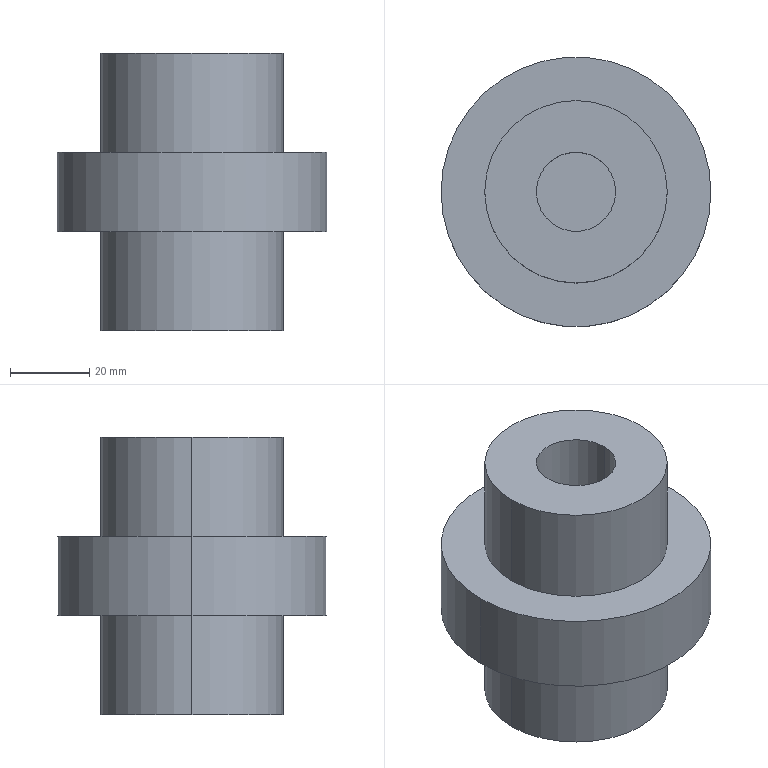Part | SolidWorks | features ICE 3, Extrusion 1, MirrorPattern 1 | 1 solid | 16 faces | box 68 x 68 x 70 mm | volume 136716 mm3 | cylinder 10 | plane 6 | commonest cylinder face diameters 46 x4 20 x2 32 x2 68 x2
STEP:
#1=CARTESIAN_POINT('',(16.,0.,-18.));
#2=VERTEX_POINT('',#1);
#3=CARTESIAN_POINT('',(-16.,0.,-18.));
#4=VERTEX_POINT('',#3);
#5=CARTESIAN_POINT('',(0.,0.,-18.));
#6=DIRECTION('',(0.,0.,-1.));
#7=DIRECTION('',(-1.,0.,0.));
#8=AXIS2_PLACEMENT_3D('',#5,#6,#7);
#9=CIRCLE('',#8,16.);
#10=EDGE_CURVE('',#2,#4,#9,.T.);
#11=ORIENTED_EDGE('',*,*,#10,.F.);
#12=CARTESIAN_POINT('',(16.,0.,-35.));
#13=VERTEX_POINT('',#12);
#14=CARTESIAN_POINT('',(16.,0.,-18.));
#15=DIRECTION('',(0.,0.,-1.));
#16=VECTOR('',#15,1000.);
#17=LINE('',#14,#16);
#18=EDGE_CURVE('',#2,#13,#17,.T.);
#19=ORIENTED_EDGE('',*,*,#18,.T.);
#20=CARTESIAN_POINT('',(-16.,0.,-35.));
#21=VERTEX_POINT('',#20);
#22=CARTESIAN_POINT('',(0.,0.,-35.));
#23=DIRECTION('',(0.,0.,-1.));
#24=DIRECTION('',(-1.,0.,0.));
#25=AXIS2_PLACEMENT_3D('',#22,#23,#24);
#26=CIRCLE('',#25,16.);
#27=EDGE_CURVE('',#13,#21,#26,.T.);
#28=ORIENTED_EDGE('',*,*,#27,.T.);
#29=CARTESIAN_POINT('',(-16.,0.,-18.));
#30=DIRECTION('',(0.,0.,-1.));
#31=VECTOR('',#30,1000.);
#32=LINE('',#29,#31);
#33=EDGE_CURVE('',#4,#21,#32,.T.);
#34=ORIENTED_EDGE('',*,*,#33,.F.);
#35=EDGE_LOOP('',(#11,#19,#28,#34));
#36=FACE_OUTER_BOUND('',#35,.T.);
#37=CARTESIAN_POINT('',(0.,0.,-18.));
#38=DIRECTION('',(0.,0.,-1.));
#39=DIRECTION('',(-1.,0.,0.));
#40=AXIS2_PLACEMENT_3D('',#37,#38,#39);
#41=CYLINDRICAL_SURFACE('',#40,16.);
#42=ADVANCED_FACE('',(#36),#41,.F.);
#43=CARTESIAN_POINT('',(-10.,0.,18.));
#44=VERTEX_POINT('',#43);
#45=CARTESIAN_POINT('',(10.,0.,18.));
#46=VERTEX_POINT('',#45);
#47=CARTESIAN_POINT('',(0.,0.,18.));
#48=DIRECTION('',(0.,0.,1.));
#49=DIRECTION('',(1.,0.,0.));
#50=AXIS2_PLACEMENT_3D('',#47,#48,#49);
#51=CIRCLE('',#50,10.);
#52=EDGE_CURVE('',#44,#46,#51,.T.);
#53=ORIENTED_EDGE('',*,*,#52,.F.);
#54=CARTESIAN_POINT('',(-10.,0.,35.));
#55=VERTEX_POINT('',#54);
#56=CARTESIAN_POINT('',(-10.,0.,18.));
#57=DIRECTION('',(0.,0.,1.));
#58=VECTOR('',#57,1000.);
#59=LINE('',#56,#58);
#60=EDGE_CURVE('',#44,#55,#59,.T.);
#61=ORIENTED_EDGE('',*,*,#60,.T.);
#62=CARTESIAN_POINT('',(10.,0.,35.));
#63=VERTEX_POINT('',#62);
#64=CARTESIAN_POINT('',(0.,0.,35.));
#65=DIRECTION('',(0.,0.,1.));
#66=DIRECTION('',(1.,0.,0.));
#67=AXIS2_PLACEMENT_3D('',#64,#65,#66);
#68=CIRCLE('',#67,10.);
#69=EDGE_CURVE('',#55,#63,#68,.T.);
#70=ORIENTED_EDGE('',*,*,#69,.T.);
#71=CARTESIAN_POINT('',(10.,0.,18.));
#72=DIRECTION('',(0.,0.,1.));
#73=VECTOR('',#72,1000.);
#74=LINE('',#71,#73);
#75=EDGE_CURVE('',#46,#63,#74,.T.);
#76=ORIENTED_EDGE('',*,*,#75,.F.);
#77=EDGE_LOOP('',(#53,#61,#70,#76));
#78=FACE_OUTER_BOUND('',#77,.T.);
#79=CARTESIAN_POINT('',(0.,0.,18.));
#80=DIRECTION('',(0.,0.,1.));
#81=DIRECTION('',(1.,0.,0.));
#82=AXIS2_PLACEMENT_3D('',#79,#80,#81);
#83=CYLINDRICAL_SURFACE('',#82,10.);
#84=ADVANCED_FACE('',(#78),#83,.F.);
#85=CARTESIAN_POINT('',(23.,0.,-35.));
#86=VERTEX_POINT('',#85);
#87=CARTESIAN_POINT('',(-23.,0.,-35.));
#88=VERTEX_POINT('',#87);
#89=CARTESIAN_POINT('',(0.,0.,-35.));
#90=DIRECTION('',(0.,0.,1.));
#91=DIRECTION('',(1.,0.,0.));
#92=AXIS2_PLACEMENT_3D('',#89,#90,#91);
#93=CIRCLE('',#92,23.);
#94=EDGE_CURVE('',#86,#88,#93,.T.);
#95=ORIENTED_EDGE('',*,*,#94,.T.);
#96=CARTESIAN_POINT('',(-23.,0.,-10.));
#97=VERTEX_POINT('',#96);
#98=CARTESIAN_POINT('',(-23.,0.,-35.));
#99=DIRECTION('',(0.,0.,1.));
#100=VECTOR('',#99,1000.);
#101=LINE('',#98,#100);
#102=EDGE_CURVE('',#88,#97,#101,.T.);
#103=ORIENTED_EDGE('',*,*,#102,.T.);
#104=CARTESIAN_POINT('',(23.,0.,-10.));
#105=VERTEX_POINT('',#104);
#106=CARTESIAN_POINT('',(0.,0.,-10.));
#107=DIRECTION('',(0.,0.,1.));
#108=DIRECTION('',(1.,0.,0.));
#109=AXIS2_PLACEMENT_3D('',#106,#107,#108);
#110=CIRCLE('',#109,23.);
#111=EDGE_CURVE('',#105,#97,#110,.T.);
#112=ORIENTED_EDGE('',*,*,#111,.F.);
#113=CARTESIAN_POINT('',(23.,0.,-35.));
#114=DIRECTION('',(0.,0.,1.));
#115=VECTOR('',#114,1000.);
#116=LINE('',#113,#115);
#117=EDGE_CURVE('',#86,#105,#116,.T.);
#118=ORIENTED_EDGE('',*,*,#117,.F.);
#119=EDGE_LOOP('',(#95,#103,#112,#118));
#120=FACE_OUTER_BOUND('',#119,.T.);
#121=CARTESIAN_POINT('',(0.,0.,-35.));
#122=DIRECTION('',(0.,0.,1.));
#123=DIRECTION('',(1.,0.,0.));
#124=AXIS2_PLACEMENT_3D('',#121,#122,#123);
#125=CYLINDRICAL_SURFACE('',#124,23.);
#126=ADVANCED_FACE('',(#120),#125,.T.);
#127=CARTESIAN_POINT('',(23.,0.,35.));
#128=VERTEX_POINT('',#127);
#129=CARTESIAN_POINT('',(-23.,0.,35.));
#130=VERTEX_POINT('',#129);
#131=CARTESIAN_POINT('',(0.,0.,35.));
#132=DIRECTION('',(0.,0.,1.));
#133=DIRECTION('',(1.,0.,0.));
#134=AXIS2_PLACEMENT_3D('',#131,#132,#133);
#135=CIRCLE('',#134,23.);
#136=EDGE_CURVE('',#128,#130,#135,.T.);
#137=ORIENTED_EDGE('',*,*,#136,.F.);
#138=CARTESIAN_POINT('',(23.,0.,10.));
#139=VERTEX_POINT('',#138);
#140=CARTESIAN_POINT('',(23.,0.,35.));
#141=DIRECTION('',(0.,0.,-1.));
#142=VECTOR('',#141,1000.);
#143=LINE('',#140,#142);
#144=EDGE_CURVE('',#128,#139,#143,.T.);
#145=ORIENTED_EDGE('',*,*,#144,.T.);
#146=CARTESIAN_POINT('',(-23.,0.,10.));
#147=VERTEX_POINT('',#146);
#148=CARTESIAN_POINT('',(0.,0.,10.));
#149=DIRECTION('',(0.,0.,1.));
#150=DIRECTION('',(1.,0.,0.));
#151=AXIS2_PLACEMENT_3D('',#148,#149,#150);
#152=CIRCLE('',#151,23.);
#153=EDGE_CURVE('',#139,#147,#152,.T.);
#154=ORIENTED_EDGE('',*,*,#153,.T.);
#155=CARTESIAN_POINT('',(-23.,0.,35.));
#156=DIRECTION('',(0.,0.,-1.));
#157=VECTOR('',#156,1000.);
#158=LINE('',#155,#157);
#159=EDGE_CURVE('',#130,#147,#158,.T.);
#160=ORIENTED_EDGE('',*,*,#159,.F.);
#161=EDGE_LOOP('',(#137,#145,#154,#160));
#162=FACE_OUTER_BOUND('',#161,.T.);
#163=CARTESIAN_POINT('',(0.,0.,35.));
#164=DIRECTION('',(0.,0.,-1.));
#165=DIRECTION('',(-1.,0.,0.));
#166=AXIS2_PLACEMENT_3D('',#163,#164,#165);
#167=CYLINDRICAL_SURFACE('',#166,23.);
#168=ADVANCED_FACE('',(#162),#167,.T.);
#169=CARTESIAN_POINT('',(34.,0.,10.));
#170=VERTEX_POINT('',#169);
#171=CARTESIAN_POINT('',(-34.,0.,10.));
#172=VERTEX_POINT('',#171);
#173=CARTESIAN_POINT('',(0.,0.,10.));
#174=DIRECTION('',(0.,0.,1.));
#175=DIRECTION('',(1.,0.,0.));
#176=AXIS2_PLACEMENT_3D('',#173,#174,#175);
#177=CIRCLE('',#176,34.);
#178=EDGE_CURVE('',#170,#172,#177,.T.);
#179=ORIENTED_EDGE('',*,*,#178,.F.);
#180=CARTESIAN_POINT('',(34.,0.,-10.));
#181=VERTEX_POINT('',#180);
#182=CARTESIAN_POINT('',(34.,0.,10.));
#183=DIRECTION('',(0.,0.,-1.));
#184=VECTOR('',#183,1000.);
#185=LINE('',#182,#184);
#186=EDGE_CURVE('',#170,#181,#185,.T.);
#187=ORIENTED_EDGE('',*,*,#186,.T.);
#188=CARTESIAN_POINT('',(-34.,0.,-10.));
#189=VERTEX_POINT('',#188);
#190=CARTESIAN_POINT('',(0.,0.,-10.));
#191=DIRECTION('',(0.,0.,1.));
#192=DIRECTION('',(1.,0.,0.));
#193=AXIS2_PLACEMENT_3D('',#190,#191,#192);
#194=CIRCLE('',#193,34.);
#195=EDGE_CURVE('',#181,#189,#194,.T.);
#196=ORIENTED_EDGE('',*,*,#195,.T.);
#197=CARTESIAN_POINT('',(-34.,0.,10.));
#198=DIRECTION('',(0.,0.,-1.));
#199=VECTOR('',#198,1000.);
#200=LINE('',#197,#199);
#201=EDGE_CURVE('',#172,#189,#200,.T.);
#202=ORIENTED_EDGE('',*,*,#201,.F.);
#203=EDGE_LOOP('',(#179,#187,#196,#202));
#204=FACE_OUTER_BOUND('',#203,.T.);
#205=CARTESIAN_POINT('',(0.,0.,10.));
#206=DIRECTION('',(0.,0.,-1.));
#207=DIRECTION('',(-1.,0.,0.));
#208=AXIS2_PLACEMENT_3D('',#205,#206,#207);
#209=CYLINDRICAL_SURFACE('',#208,34.);
#210=ADVANCED_FACE('',(#204),#209,.T.);
#211=CARTESIAN_POINT('',(0.,0.,10.));
#212=DIRECTION('',(0.,0.,1.));
#213=DIRECTION('',(1.,0.,0.));
#214=AXIS2_PLACEMENT_3D('',#211,#212,#213);
#215=CIRCLE('',#214,34.);
#216=EDGE_CURVE('',#172,#170,#215,.T.);
#217=ORIENTED_EDGE('',*,*,#216,.T.);
#218=ORIENTED_EDGE('',*,*,#178,.T.);
#219=EDGE_LOOP('',(#217,#218));
#220=FACE_OUTER_BOUND('',#219,.T.);
#221=CARTESIAN_POINT('',(0.,0.,10.));
#222=DIRECTION('',(0.,0.,1.));
#223=DIRECTION('',(1.,0.,0.));
#224=AXIS2_PLACEMENT_3D('',#221,#222,#223);
#225=CIRCLE('',#224,23.);
#226=EDGE_CURVE('',#147,#139,#225,.T.);
#227=ORIENTED_EDGE('',*,*,#226,.F.);
#228=ORIENTED_EDGE('',*,*,#153,.F.);
#229=EDGE_LOOP('',(#227,#228));
#230=FACE_BOUND('',#229,.T.);
#231=CARTESIAN_POINT('',(0.,0.,10.));
#232=DIRECTION('',(0.,0.,1.));
#233=DIRECTION('',(1.,0.,0.));
#234=AXIS2_PLACEMENT_3D('',#231,#232,#233);
#235=PLANE('',#234);
#236=ADVANCED_FACE('',(#220,#230),#235,.T.);
#237=ORIENTED_EDGE('',*,*,#186,.F.);
#238=ORIENTED_EDGE('',*,*,#216,.F.);
#239=ORIENTED_EDGE('',*,*,#201,.T.);
#240=CARTESIAN_POINT('',(0.,0.,-10.));
#241=DIRECTION('',(0.,0.,1.));
#242=DIRECTION('',(1.,0.,0.));
#243=AXIS2_PLACEMENT_3D('',#240,#241,#242);
#244=CIRCLE('',#243,34.);
#245=EDGE_CURVE('',#189,#181,#244,.T.);
#246=ORIENTED_EDGE('',*,*,#245,.T.);
#247=EDGE_LOOP('',(#237,#238,#239,#246));
#248=FACE_OUTER_BOUND('',#247,.T.);
#249=CARTESIAN_POINT('',(0.,0.,10.));
#250=DIRECTION('',(0.,0.,-1.));
#251=DIRECTION('',(-1.,0.,0.));
#252=AXIS2_PLACEMENT_3D('',#249,#250,#251);
#253=CYLINDRICAL_SURFACE('',#252,34.);
#254=ADVANCED_FACE('',(#248),#253,.T.);
#255=ORIENTED_EDGE('',*,*,#111,.T.);
#256=CARTESIAN_POINT('',(0.,0.,-10.));
#257=DIRECTION('',(0.,0.,1.));
#258=DIRECTION('',(1.,0.,0.));
#259=AXIS2_PLACEMENT_3D('',#256,#257,#258);
#260=CIRCLE('',#259,23.);
#261=EDGE_CURVE('',#97,#105,#260,.T.);
#262=ORIENTED_EDGE('',*,*,#261,.T.);
#263=EDGE_LOOP('',(#255,#262));
#264=FACE_BOUND('',#263,.T.);
#265=ORIENTED_EDGE('',*,*,#245,.F.);
#266=ORIENTED_EDGE('',*,*,#195,.F.);
#267=EDGE_LOOP('',(#265,#266));
#268=FACE_OUTER_BOUND('',#267,.T.);
#269=CARTESIAN_POINT('',(0.,0.,-10.));
#270=DIRECTION('',(0.,0.,1.));
#271=DIRECTION('',(1.,0.,0.));
#272=AXIS2_PLACEMENT_3D('',#269,#270,#271);
#273=PLANE('',#272);
#274=ADVANCED_FACE('',(#264,#268),#273,.F.);
#275=ORIENTED_EDGE('',*,*,#144,.F.);
#276=CARTESIAN_POINT('',(0.,0.,35.));
#277=DIRECTION('',(0.,0.,1.));
#278=DIRECTION('',(1.,0.,0.));
#279=AXIS2_PLACEMENT_3D('',#276,#277,#278);
#280=CIRCLE('',#279,23.);
#281=EDGE_CURVE('',#130,#128,#280,.T.);
#282=ORIENTED_EDGE('',*,*,#281,.F.);
#283=ORIENTED_EDGE('',*,*,#159,.T.);
#284=ORIENTED_EDGE('',*,*,#226,.T.);
#285=EDGE_LOOP('',(#275,#282,#283,#284));
#286=FACE_OUTER_BOUND('',#285,.T.);
#287=CARTESIAN_POINT('',(0.,0.,35.));
#288=DIRECTION('',(0.,0.,-1.));
#289=DIRECTION('',(-1.,0.,0.));
#290=AXIS2_PLACEMENT_3D('',#287,#288,#289);
#291=CYLINDRICAL_SURFACE('',#290,23.);
#292=ADVANCED_FACE('',(#286),#291,.T.);
#293=CARTESIAN_POINT('',(0.,0.,35.));
#294=DIRECTION('',(0.,0.,1.));
#295=DIRECTION('',(1.,0.,0.));
#296=AXIS2_PLACEMENT_3D('',#293,#294,#295);
#297=CIRCLE('',#296,10.);
#298=EDGE_CURVE('',#63,#55,#297,.T.);
#299=ORIENTED_EDGE('',*,*,#298,.F.);
#300=ORIENTED_EDGE('',*,*,#69,.F.);
#301=EDGE_LOOP('',(#299,#300));
#302=FACE_BOUND('',#301,.T.);
#303=ORIENTED_EDGE('',*,*,#281,.T.);
#304=ORIENTED_EDGE('',*,*,#136,.T.);
#305=EDGE_LOOP('',(#303,#304));
#306=FACE_OUTER_BOUND('',#305,.T.);
#307=CARTESIAN_POINT('',(0.,0.,35.));
#308=DIRECTION('',(0.,0.,1.));
#309=DIRECTION('',(1.,0.,0.));
#310=AXIS2_PLACEMENT_3D('',#307,#308,#309);
#311=PLANE('',#310);
#312=ADVANCED_FACE('',(#302,#306),#311,.T.);
#313=ORIENTED_EDGE('',*,*,#102,.F.);
#314=CARTESIAN_POINT('',(0.,0.,-35.));
#315=DIRECTION('',(0.,0.,1.));
#316=DIRECTION('',(1.,0.,0.));
#317=AXIS2_PLACEMENT_3D('',#314,#315,#316);
#318=CIRCLE('',#317,23.);
#319=EDGE_CURVE('',#88,#86,#318,.T.);
#320=ORIENTED_EDGE('',*,*,#319,.T.);
#321=ORIENTED_EDGE('',*,*,#117,.T.);
#322=ORIENTED_EDGE('',*,*,#261,.F.);
#323=EDGE_LOOP('',(#313,#320,#321,#322));
#324=FACE_OUTER_BOUND('',#323,.T.);
#325=CARTESIAN_POINT('',(0.,0.,-35.));
#326=DIRECTION('',(0.,0.,1.));
#327=DIRECTION('',(1.,0.,0.));
#328=AXIS2_PLACEMENT_3D('',#325,#326,#327);
#329=CYLINDRICAL_SURFACE('',#328,23.);
#330=ADVANCED_FACE('',(#324),#329,.T.);
#331=CARTESIAN_POINT('',(0.,0.,-35.));
#332=DIRECTION('',(0.,0.,-1.));
#333=DIRECTION('',(-1.,0.,0.));
#334=AXIS2_PLACEMENT_3D('',#331,#332,#333);
#335=CIRCLE('',#334,16.);
#336=EDGE_CURVE('',#21,#13,#335,.T.);
#337=ORIENTED_EDGE('',*,*,#336,.F.);
#338=ORIENTED_EDGE('',*,*,#27,.F.);
#339=EDGE_LOOP('',(#337,#338));
#340=FACE_BOUND('',#339,.T.);
#341=ORIENTED_EDGE('',*,*,#94,.F.);
#342=ORIENTED_EDGE('',*,*,#319,.F.);
#343=EDGE_LOOP('',(#341,#342));
#344=FACE_OUTER_BOUND('',#343,.T.);
#345=CARTESIAN_POINT('',(0.,0.,-35.));
#346=DIRECTION('',(0.,0.,-1.));
#347=DIRECTION('',(1.,0.,0.));
#348=AXIS2_PLACEMENT_3D('',#345,#346,#347);
#349=PLANE('',#348);
#350=ADVANCED_FACE('',(#340,#344),#349,.T.);
#351=ORIENTED_EDGE('',*,*,#60,.F.);
#352=CARTESIAN_POINT('',(0.,0.,18.));
#353=DIRECTION('',(0.,0.,1.));
#354=DIRECTION('',(1.,0.,0.));
#355=AXIS2_PLACEMENT_3D('',#352,#353,#354);
#356=CIRCLE('',#355,10.);
#357=EDGE_CURVE('',#46,#44,#356,.T.);
#358=ORIENTED_EDGE('',*,*,#357,.F.);
#359=ORIENTED_EDGE('',*,*,#75,.T.);
#360=ORIENTED_EDGE('',*,*,#298,.T.);
#361=EDGE_LOOP('',(#351,#358,#359,#360));
#362=FACE_OUTER_BOUND('',#361,.T.);
#363=CARTESIAN_POINT('',(0.,0.,18.));
#364=DIRECTION('',(0.,0.,1.));
#365=DIRECTION('',(1.,0.,0.));
#366=AXIS2_PLACEMENT_3D('',#363,#364,#365);
#367=CYLINDRICAL_SURFACE('',#366,10.);
#368=ADVANCED_FACE('',(#362),#367,.F.);
#369=ORIENTED_EDGE('',*,*,#357,.T.);
#370=ORIENTED_EDGE('',*,*,#52,.T.);
#371=EDGE_LOOP('',(#369,#370));
#372=FACE_OUTER_BOUND('',#371,.T.);
#373=CARTESIAN_POINT('',(0.,0.,18.));
#374=DIRECTION('',(0.,0.,1.));
#375=DIRECTION('',(1.,0.,0.));
#376=AXIS2_PLACEMENT_3D('',#373,#374,#375);
#377=PLANE('',#376);
#378=ADVANCED_FACE('',(#372),#377,.T.);
#379=ORIENTED_EDGE('',*,*,#18,.F.);
#380=CARTESIAN_POINT('',(0.,0.,-18.));
#381=DIRECTION('',(0.,0.,-1.));
#382=DIRECTION('',(-1.,0.,0.));
#383=AXIS2_PLACEMENT_3D('',#380,#381,#382);
#384=CIRCLE('',#383,16.);
#385=EDGE_CURVE('',#4,#2,#384,.T.);
#386=ORIENTED_EDGE('',*,*,#385,.F.);
#387=ORIENTED_EDGE('',*,*,#33,.T.);
#388=ORIENTED_EDGE('',*,*,#336,.T.);
#389=EDGE_LOOP('',(#379,#386,#387,#388));
#390=FACE_OUTER_BOUND('',#389,.T.);
#391=CARTESIAN_POINT('',(0.,0.,-18.));
#392=DIRECTION('',(0.,0.,-1.));
#393=DIRECTION('',(-1.,0.,0.));
#394=AXIS2_PLACEMENT_3D('',#391,#392,#393);
#395=CYLINDRICAL_SURFACE('',#394,16.);
#396=ADVANCED_FACE('',(#390),#395,.F.);
#397=ORIENTED_EDGE('',*,*,#385,.T.);
#398=ORIENTED_EDGE('',*,*,#10,.T.);
#399=EDGE_LOOP('',(#397,#398));
#400=FACE_OUTER_BOUND('',#399,.T.);
#401=CARTESIAN_POINT('',(0.,0.,-18.));
#402=DIRECTION('',(0.,0.,-1.));
#403=DIRECTION('',(-1.,0.,0.));
#404=AXIS2_PLACEMENT_3D('',#401,#402,#403);
#405=PLANE('',#404);
#406=ADVANCED_FACE('',(#400),#405,.T.);
#407=CLOSED_SHELL('',(#42,#84,#126,#168,#210,#236,#254,#274,#292,#312,#330,#350,#368,#378,#396,#406));
#408=MANIFOLD_SOLID_BREP('',#407);
#409=CARTESIAN_POINT('',(0.,0.,0.));
#410=DIRECTION('',(0.,0.,1.));
#411=DIRECTION('',(1.,0.,0.));
#412=AXIS2_PLACEMENT_3D('',#409,#410,#411);
#413=(LENGTH_UNIT()NAMED_UNIT(*)SI_UNIT(.MILLI.,.METRE.));
#414=UNCERTAINTY_MEASURE_WITH_UNIT(LENGTH_MEASURE(0.00001),#413,'','');
#415=(NAMED_UNIT(*)PLANE_ANGLE_UNIT()SI_UNIT($,.RADIAN.));
#416=(NAMED_UNIT(*)SI_UNIT($,.STERADIAN.)SOLID_ANGLE_UNIT());
#417=(GEOMETRIC_REPRESENTATION_CONTEXT(3)GLOBAL_UNCERTAINTY_ASSIGNED_CONTEXT((#414))GLOBAL_UNIT_ASSIGNED_CONTEXT((#413,#415,#416))REPRESENTATION_CONTEXT('',''));
#418=ADVANCED_BREP_SHAPE_REPRESENTATION('',(#408,#412),#417);